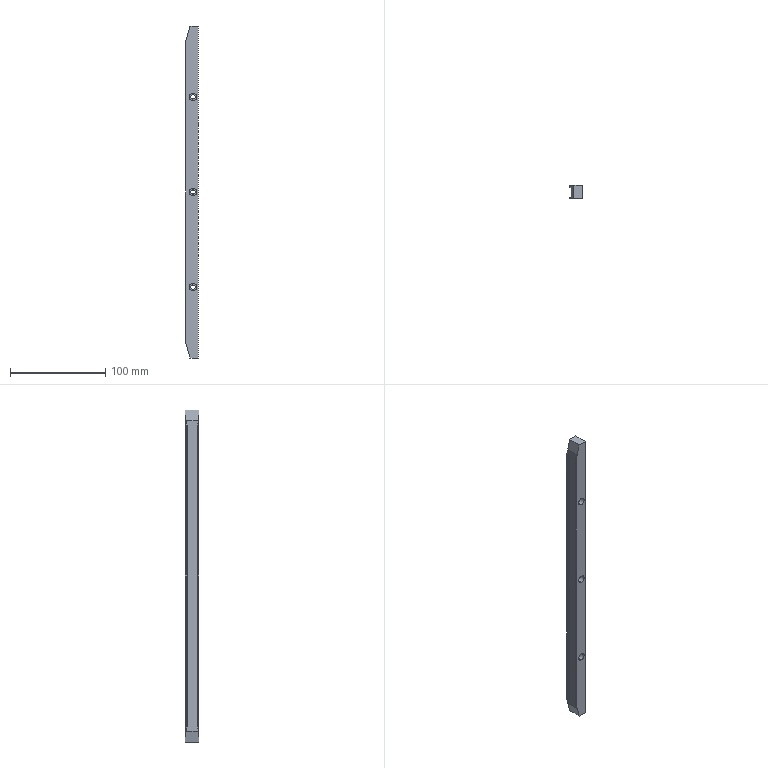Part | STEP file | 1 solid | 33 faces | box 13.5 x 14 x 349 mm | volume 58115 mm3 | plane 21 | cylinder 12 | commonest cylinder face diameters 4.5 x6 8 x6